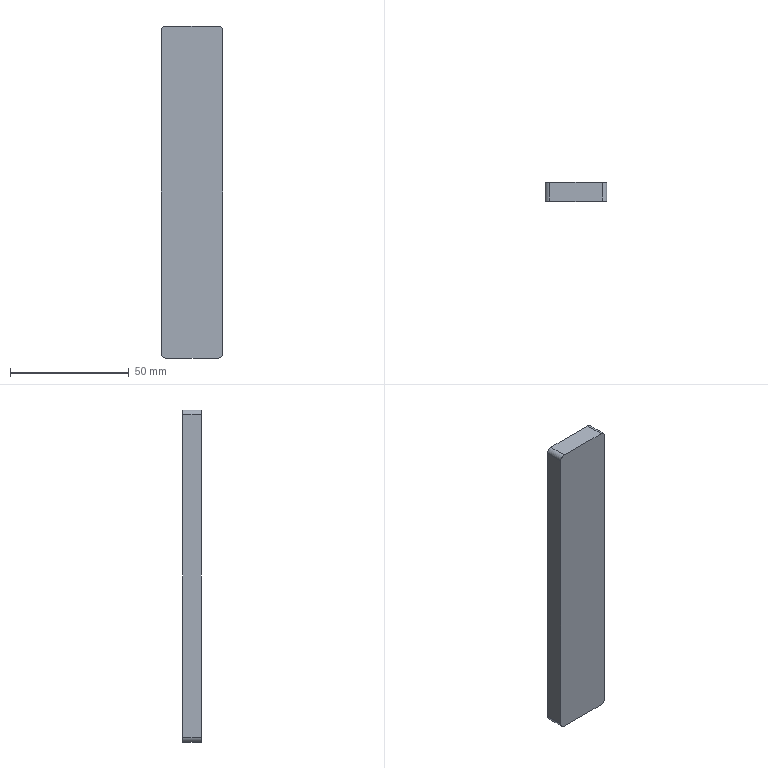Part | SolidWorks | features Fillet 1, FlatPattern 1, SMBaseFlange 1, SheetMetal 1 | 1 solid | 10 faces | box 26 x 8 x 140 mm | volume 29093 mm3 | plane 6 | cylinder 4 | commonest cylinder face diameters 4 x4
STEP:
#1=CARTESIAN_POINT('',(13.,8.,68.));
#2=VERTEX_POINT('',#1);
#3=CARTESIAN_POINT('',(13.,8.,-68.));
#4=VERTEX_POINT('',#3);
#5=CARTESIAN_POINT('',(13.,8.,-70.));
#6=DIRECTION('',(0.,0.,-1.));
#7=VECTOR('',#6,1000.);
#8=LINE('',#5,#7);
#9=EDGE_CURVE('',#2,#4,#8,.T.);
#10=ORIENTED_EDGE('',*,*,#9,.F.);
#11=CARTESIAN_POINT('',(13.,0.,68.));
#12=VERTEX_POINT('',#11);
#13=CARTESIAN_POINT('',(13.,8.,68.));
#14=DIRECTION('',(0.,-1.,0.));
#15=VECTOR('',#14,1000.);
#16=LINE('',#13,#15);
#17=EDGE_CURVE('',#2,#12,#16,.T.);
#18=ORIENTED_EDGE('',*,*,#17,.T.);
#19=CARTESIAN_POINT('',(13.,0.,-68.));
#20=VERTEX_POINT('',#19);
#21=CARTESIAN_POINT('',(13.,0.,-70.));
#22=DIRECTION('',(0.,0.,-1.));
#23=VECTOR('',#22,1000.);
#24=LINE('',#21,#23);
#25=EDGE_CURVE('',#12,#20,#24,.T.);
#26=ORIENTED_EDGE('',*,*,#25,.T.);
#27=CARTESIAN_POINT('',(13.,8.,-68.));
#28=DIRECTION('',(0.,1.,0.));
#29=VECTOR('',#28,1000.);
#30=LINE('',#27,#29);
#31=EDGE_CURVE('',#20,#4,#30,.T.);
#32=ORIENTED_EDGE('',*,*,#31,.T.);
#33=EDGE_LOOP('',(#10,#18,#26,#32));
#34=FACE_OUTER_BOUND('',#33,.T.);
#35=CARTESIAN_POINT('',(13.,8.,-70.));
#36=DIRECTION('',(-1.,0.,0.));
#37=DIRECTION('',(0.,0.,1.));
#38=AXIS2_PLACEMENT_3D('',#35,#36,#37);
#39=PLANE('',#38);
#40=ADVANCED_FACE('',(#34),#39,.F.);
#41=CARTESIAN_POINT('',(11.,8.,-70.));
#42=VERTEX_POINT('',#41);
#43=CARTESIAN_POINT('',(-11.,8.,-70.));
#44=VERTEX_POINT('',#43);
#45=CARTESIAN_POINT('',(-13.,8.,-70.));
#46=DIRECTION('',(-1.,0.,0.));
#47=VECTOR('',#46,1000.);
#48=LINE('',#45,#47);
#49=EDGE_CURVE('',#42,#44,#48,.T.);
#50=ORIENTED_EDGE('',*,*,#49,.F.);
#51=CARTESIAN_POINT('',(11.,0.,-70.));
#52=VERTEX_POINT('',#51);
#53=CARTESIAN_POINT('',(11.,8.,-70.));
#54=DIRECTION('',(0.,-1.,0.));
#55=VECTOR('',#54,1000.);
#56=LINE('',#53,#55);
#57=EDGE_CURVE('',#42,#52,#56,.T.);
#58=ORIENTED_EDGE('',*,*,#57,.T.);
#59=CARTESIAN_POINT('',(-11.,0.,-70.));
#60=VERTEX_POINT('',#59);
#61=CARTESIAN_POINT('',(-13.,0.,-70.));
#62=DIRECTION('',(-1.,0.,0.));
#63=VECTOR('',#62,1000.);
#64=LINE('',#61,#63);
#65=EDGE_CURVE('',#52,#60,#64,.T.);
#66=ORIENTED_EDGE('',*,*,#65,.T.);
#67=CARTESIAN_POINT('',(-11.,8.,-70.));
#68=DIRECTION('',(0.,1.,0.));
#69=VECTOR('',#68,1000.);
#70=LINE('',#67,#69);
#71=EDGE_CURVE('',#60,#44,#70,.T.);
#72=ORIENTED_EDGE('',*,*,#71,.T.);
#73=EDGE_LOOP('',(#50,#58,#66,#72));
#74=FACE_OUTER_BOUND('',#73,.T.);
#75=CARTESIAN_POINT('',(-13.,8.,-70.));
#76=DIRECTION('',(0.,0.,1.));
#77=DIRECTION('',(1.,0.,0.));
#78=AXIS2_PLACEMENT_3D('',#75,#76,#77);
#79=PLANE('',#78);
#80=ADVANCED_FACE('',(#74),#79,.F.);
#81=CARTESIAN_POINT('',(-13.,0.,-68.));
#82=VERTEX_POINT('',#81);
#83=CARTESIAN_POINT('',(-13.,0.,68.));
#84=VERTEX_POINT('',#83);
#85=CARTESIAN_POINT('',(-13.,0.,-70.));
#86=DIRECTION('',(0.,0.,1.));
#87=VECTOR('',#86,1000.);
#88=LINE('',#85,#87);
#89=EDGE_CURVE('',#82,#84,#88,.T.);
#90=ORIENTED_EDGE('',*,*,#89,.T.);
#91=CARTESIAN_POINT('',(-13.,8.,68.));
#92=VERTEX_POINT('',#91);
#93=CARTESIAN_POINT('',(-13.,8.,68.));
#94=DIRECTION('',(0.,1.,0.));
#95=VECTOR('',#94,1000.);
#96=LINE('',#93,#95);
#97=EDGE_CURVE('',#84,#92,#96,.T.);
#98=ORIENTED_EDGE('',*,*,#97,.T.);
#99=CARTESIAN_POINT('',(-13.,8.,-68.));
#100=VERTEX_POINT('',#99);
#101=CARTESIAN_POINT('',(-13.,8.,-70.));
#102=DIRECTION('',(0.,0.,1.));
#103=VECTOR('',#102,1000.);
#104=LINE('',#101,#103);
#105=EDGE_CURVE('',#100,#92,#104,.T.);
#106=ORIENTED_EDGE('',*,*,#105,.F.);
#107=CARTESIAN_POINT('',(-13.,8.,-68.));
#108=DIRECTION('',(0.,-1.,0.));
#109=VECTOR('',#108,1000.);
#110=LINE('',#107,#109);
#111=EDGE_CURVE('',#100,#82,#110,.T.);
#112=ORIENTED_EDGE('',*,*,#111,.T.);
#113=EDGE_LOOP('',(#90,#98,#106,#112));
#114=FACE_OUTER_BOUND('',#113,.T.);
#115=CARTESIAN_POINT('',(-13.,8.,-70.));
#116=DIRECTION('',(1.,0.,0.));
#117=DIRECTION('',(0.,0.,-1.));
#118=AXIS2_PLACEMENT_3D('',#115,#116,#117);
#119=PLANE('',#118);
#120=ADVANCED_FACE('',(#114),#119,.F.);
#121=CARTESIAN_POINT('',(-11.,8.,70.));
#122=VERTEX_POINT('',#121);
#123=CARTESIAN_POINT('',(11.,8.,70.));
#124=VERTEX_POINT('',#123);
#125=CARTESIAN_POINT('',(-13.,8.,70.));
#126=DIRECTION('',(1.,0.,0.));
#127=VECTOR('',#126,1000.);
#128=LINE('',#125,#127);
#129=EDGE_CURVE('',#122,#124,#128,.T.);
#130=ORIENTED_EDGE('',*,*,#129,.F.);
#131=CARTESIAN_POINT('',(-11.,0.,70.));
#132=VERTEX_POINT('',#131);
#133=CARTESIAN_POINT('',(-11.,8.,70.));
#134=DIRECTION('',(0.,-1.,0.));
#135=VECTOR('',#134,1000.);
#136=LINE('',#133,#135);
#137=EDGE_CURVE('',#122,#132,#136,.T.);
#138=ORIENTED_EDGE('',*,*,#137,.T.);
#139=CARTESIAN_POINT('',(11.,0.,70.));
#140=VERTEX_POINT('',#139);
#141=CARTESIAN_POINT('',(-13.,0.,70.));
#142=DIRECTION('',(1.,0.,0.));
#143=VECTOR('',#142,1000.);
#144=LINE('',#141,#143);
#145=EDGE_CURVE('',#132,#140,#144,.T.);
#146=ORIENTED_EDGE('',*,*,#145,.T.);
#147=CARTESIAN_POINT('',(11.,8.,70.));
#148=DIRECTION('',(0.,1.,0.));
#149=VECTOR('',#148,1000.);
#150=LINE('',#147,#149);
#151=EDGE_CURVE('',#140,#124,#150,.T.);
#152=ORIENTED_EDGE('',*,*,#151,.T.);
#153=EDGE_LOOP('',(#130,#138,#146,#152));
#154=FACE_OUTER_BOUND('',#153,.T.);
#155=CARTESIAN_POINT('',(-13.,8.,70.));
#156=DIRECTION('',(0.,0.,-1.));
#157=DIRECTION('',(-1.,0.,0.));
#158=AXIS2_PLACEMENT_3D('',#155,#156,#157);
#159=PLANE('',#158);
#160=ADVANCED_FACE('',(#154),#159,.F.);
#161=ORIENTED_EDGE('',*,*,#105,.T.);
#162=CARTESIAN_POINT('',(-11.,8.,68.));
#163=DIRECTION('',(0.,1.,0.));
#164=DIRECTION('',(0.,0.,1.));
#165=AXIS2_PLACEMENT_3D('',#162,#163,#164);
#166=CIRCLE('',#165,2.);
#167=EDGE_CURVE('',#92,#122,#166,.T.);
#168=ORIENTED_EDGE('',*,*,#167,.T.);
#169=ORIENTED_EDGE('',*,*,#129,.T.);
#170=CARTESIAN_POINT('',(11.,8.,68.));
#171=DIRECTION('',(0.,1.,0.));
#172=DIRECTION('',(0.,0.,1.));
#173=AXIS2_PLACEMENT_3D('',#170,#171,#172);
#174=CIRCLE('',#173,2.);
#175=EDGE_CURVE('',#124,#2,#174,.T.);
#176=ORIENTED_EDGE('',*,*,#175,.T.);
#177=ORIENTED_EDGE('',*,*,#9,.T.);
#178=CARTESIAN_POINT('',(11.,8.,-68.));
#179=DIRECTION('',(0.,1.,0.));
#180=DIRECTION('',(0.,0.,1.));
#181=AXIS2_PLACEMENT_3D('',#178,#179,#180);
#182=CIRCLE('',#181,2.);
#183=EDGE_CURVE('',#4,#42,#182,.T.);
#184=ORIENTED_EDGE('',*,*,#183,.T.);
#185=ORIENTED_EDGE('',*,*,#49,.T.);
#186=CARTESIAN_POINT('',(-11.,8.,-68.));
#187=DIRECTION('',(0.,1.,0.));
#188=DIRECTION('',(0.,0.,1.));
#189=AXIS2_PLACEMENT_3D('',#186,#187,#188);
#190=CIRCLE('',#189,2.);
#191=EDGE_CURVE('',#44,#100,#190,.T.);
#192=ORIENTED_EDGE('',*,*,#191,.T.);
#193=EDGE_LOOP('',(#161,#168,#169,#176,#177,#184,#185,#192));
#194=FACE_OUTER_BOUND('',#193,.T.);
#195=CARTESIAN_POINT('',(0.,8.,0.));
#196=DIRECTION('',(0.,1.,0.));
#197=DIRECTION('',(0.,0.,1.));
#198=AXIS2_PLACEMENT_3D('',#195,#196,#197);
#199=PLANE('',#198);
#200=ADVANCED_FACE('',(#194),#199,.T.);
#201=ORIENTED_EDGE('',*,*,#145,.F.);
#202=CARTESIAN_POINT('',(-11.,0.,68.));
#203=DIRECTION('',(0.,-1.,0.));
#204=DIRECTION('',(0.,0.,1.));
#205=AXIS2_PLACEMENT_3D('',#202,#203,#204);
#206=CIRCLE('',#205,2.);
#207=EDGE_CURVE('',#132,#84,#206,.T.);
#208=ORIENTED_EDGE('',*,*,#207,.T.);
#209=ORIENTED_EDGE('',*,*,#89,.F.);
#210=CARTESIAN_POINT('',(-11.,0.,-68.));
#211=DIRECTION('',(0.,-1.,0.));
#212=DIRECTION('',(0.,0.,1.));
#213=AXIS2_PLACEMENT_3D('',#210,#211,#212);
#214=CIRCLE('',#213,2.);
#215=EDGE_CURVE('',#82,#60,#214,.T.);
#216=ORIENTED_EDGE('',*,*,#215,.T.);
#217=ORIENTED_EDGE('',*,*,#65,.F.);
#218=CARTESIAN_POINT('',(11.,0.,-68.));
#219=DIRECTION('',(0.,-1.,0.));
#220=DIRECTION('',(0.,0.,1.));
#221=AXIS2_PLACEMENT_3D('',#218,#219,#220);
#222=CIRCLE('',#221,2.);
#223=EDGE_CURVE('',#52,#20,#222,.T.);
#224=ORIENTED_EDGE('',*,*,#223,.T.);
#225=ORIENTED_EDGE('',*,*,#25,.F.);
#226=CARTESIAN_POINT('',(11.,0.,68.));
#227=DIRECTION('',(0.,-1.,0.));
#228=DIRECTION('',(0.,0.,1.));
#229=AXIS2_PLACEMENT_3D('',#226,#227,#228);
#230=CIRCLE('',#229,2.);
#231=EDGE_CURVE('',#12,#140,#230,.T.);
#232=ORIENTED_EDGE('',*,*,#231,.T.);
#233=EDGE_LOOP('',(#201,#208,#209,#216,#217,#224,#225,#232));
#234=FACE_OUTER_BOUND('',#233,.T.);
#235=CARTESIAN_POINT('',(0.,0.,0.));
#236=DIRECTION('',(0.,1.,0.));
#237=DIRECTION('',(0.,0.,1.));
#238=AXIS2_PLACEMENT_3D('',#235,#236,#237);
#239=PLANE('',#238);
#240=ADVANCED_FACE('',(#234),#239,.F.);
#241=ORIENTED_EDGE('',*,*,#167,.F.);
#242=ORIENTED_EDGE('',*,*,#97,.F.);
#243=ORIENTED_EDGE('',*,*,#207,.F.);
#244=ORIENTED_EDGE('',*,*,#137,.F.);
#245=EDGE_LOOP('',(#241,#242,#243,#244));
#246=FACE_OUTER_BOUND('',#245,.T.);
#247=CARTESIAN_POINT('',(-11.,8.,68.));
#248=DIRECTION('',(0.,-1.,0.));
#249=DIRECTION('',(0.,0.,-1.));
#250=AXIS2_PLACEMENT_3D('',#247,#248,#249);
#251=CYLINDRICAL_SURFACE('',#250,2.);
#252=ADVANCED_FACE('',(#246),#251,.T.);
#253=ORIENTED_EDGE('',*,*,#175,.F.);
#254=ORIENTED_EDGE('',*,*,#151,.F.);
#255=ORIENTED_EDGE('',*,*,#231,.F.);
#256=ORIENTED_EDGE('',*,*,#17,.F.);
#257=EDGE_LOOP('',(#253,#254,#255,#256));
#258=FACE_OUTER_BOUND('',#257,.T.);
#259=CARTESIAN_POINT('',(11.,8.,68.));
#260=DIRECTION('',(0.,-1.,0.));
#261=DIRECTION('',(0.,0.,-1.));
#262=AXIS2_PLACEMENT_3D('',#259,#260,#261);
#263=CYLINDRICAL_SURFACE('',#262,2.);
#264=ADVANCED_FACE('',(#258),#263,.T.);
#265=ORIENTED_EDGE('',*,*,#183,.F.);
#266=ORIENTED_EDGE('',*,*,#31,.F.);
#267=ORIENTED_EDGE('',*,*,#223,.F.);
#268=ORIENTED_EDGE('',*,*,#57,.F.);
#269=EDGE_LOOP('',(#265,#266,#267,#268));
#270=FACE_OUTER_BOUND('',#269,.T.);
#271=CARTESIAN_POINT('',(11.,8.,-68.));
#272=DIRECTION('',(0.,-1.,0.));
#273=DIRECTION('',(0.,0.,-1.));
#274=AXIS2_PLACEMENT_3D('',#271,#272,#273);
#275=CYLINDRICAL_SURFACE('',#274,2.);
#276=ADVANCED_FACE('',(#270),#275,.T.);
#277=ORIENTED_EDGE('',*,*,#191,.F.);
#278=ORIENTED_EDGE('',*,*,#71,.F.);
#279=ORIENTED_EDGE('',*,*,#215,.F.);
#280=ORIENTED_EDGE('',*,*,#111,.F.);
#281=EDGE_LOOP('',(#277,#278,#279,#280));
#282=FACE_OUTER_BOUND('',#281,.T.);
#283=CARTESIAN_POINT('',(-11.,8.,-68.));
#284=DIRECTION('',(0.,-1.,0.));
#285=DIRECTION('',(0.,0.,-1.));
#286=AXIS2_PLACEMENT_3D('',#283,#284,#285);
#287=CYLINDRICAL_SURFACE('',#286,2.);
#288=ADVANCED_FACE('',(#282),#287,.T.);
#289=CLOSED_SHELL('',(#40,#80,#120,#160,#200,#240,#252,#264,#276,#288));
#290=MANIFOLD_SOLID_BREP('',#289);
#291=CARTESIAN_POINT('',(0.,0.,0.));
#292=DIRECTION('',(0.,0.,1.));
#293=DIRECTION('',(1.,0.,0.));
#294=AXIS2_PLACEMENT_3D('',#291,#292,#293);
#295=(LENGTH_UNIT()NAMED_UNIT(*)SI_UNIT(.MILLI.,.METRE.));
#296=UNCERTAINTY_MEASURE_WITH_UNIT(LENGTH_MEASURE(0.00001),#295,'','');
#297=(NAMED_UNIT(*)PLANE_ANGLE_UNIT()SI_UNIT($,.RADIAN.));
#298=(NAMED_UNIT(*)SI_UNIT($,.STERADIAN.)SOLID_ANGLE_UNIT());
#299=(GEOMETRIC_REPRESENTATION_CONTEXT(3)GLOBAL_UNCERTAINTY_ASSIGNED_CONTEXT((#296))GLOBAL_UNIT_ASSIGNED_CONTEXT((#295,#297,#298))REPRESENTATION_CONTEXT('',''));
#300=ADVANCED_BREP_SHAPE_REPRESENTATION('',(#290,#294),#299);